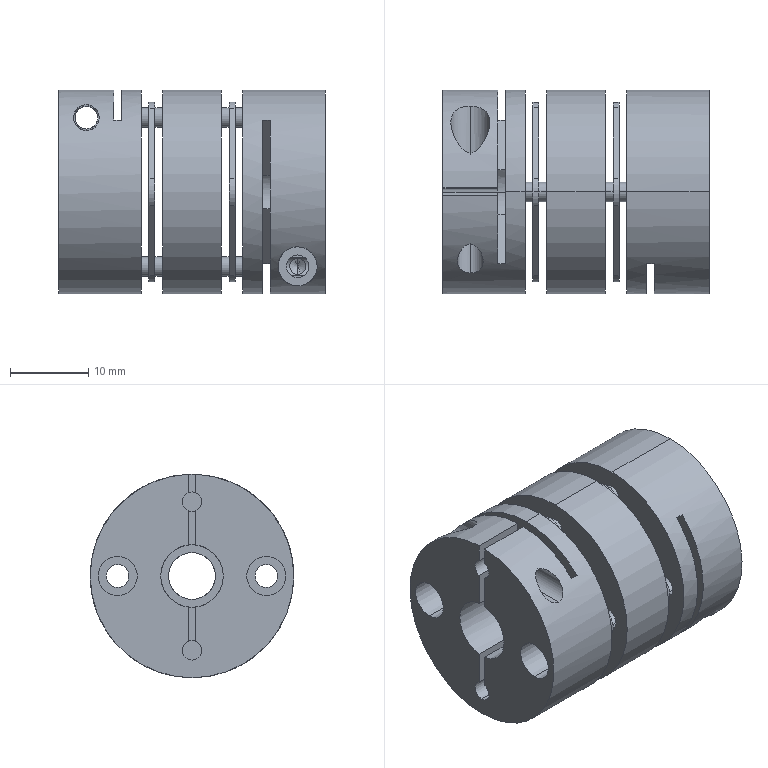Part | STEP file | Double diaphragm coupling LC-A-020DA-06B-08B | 1 solid | 149 faces | box 34 x 26 x 26 mm | volume 11838 mm3 | cylinder 97 | plane 50 | cone 2 | commonest cylinder face diameters 2.5 x31 2.9 x24 5 x22 12 x6 26 x6 2.05 x2